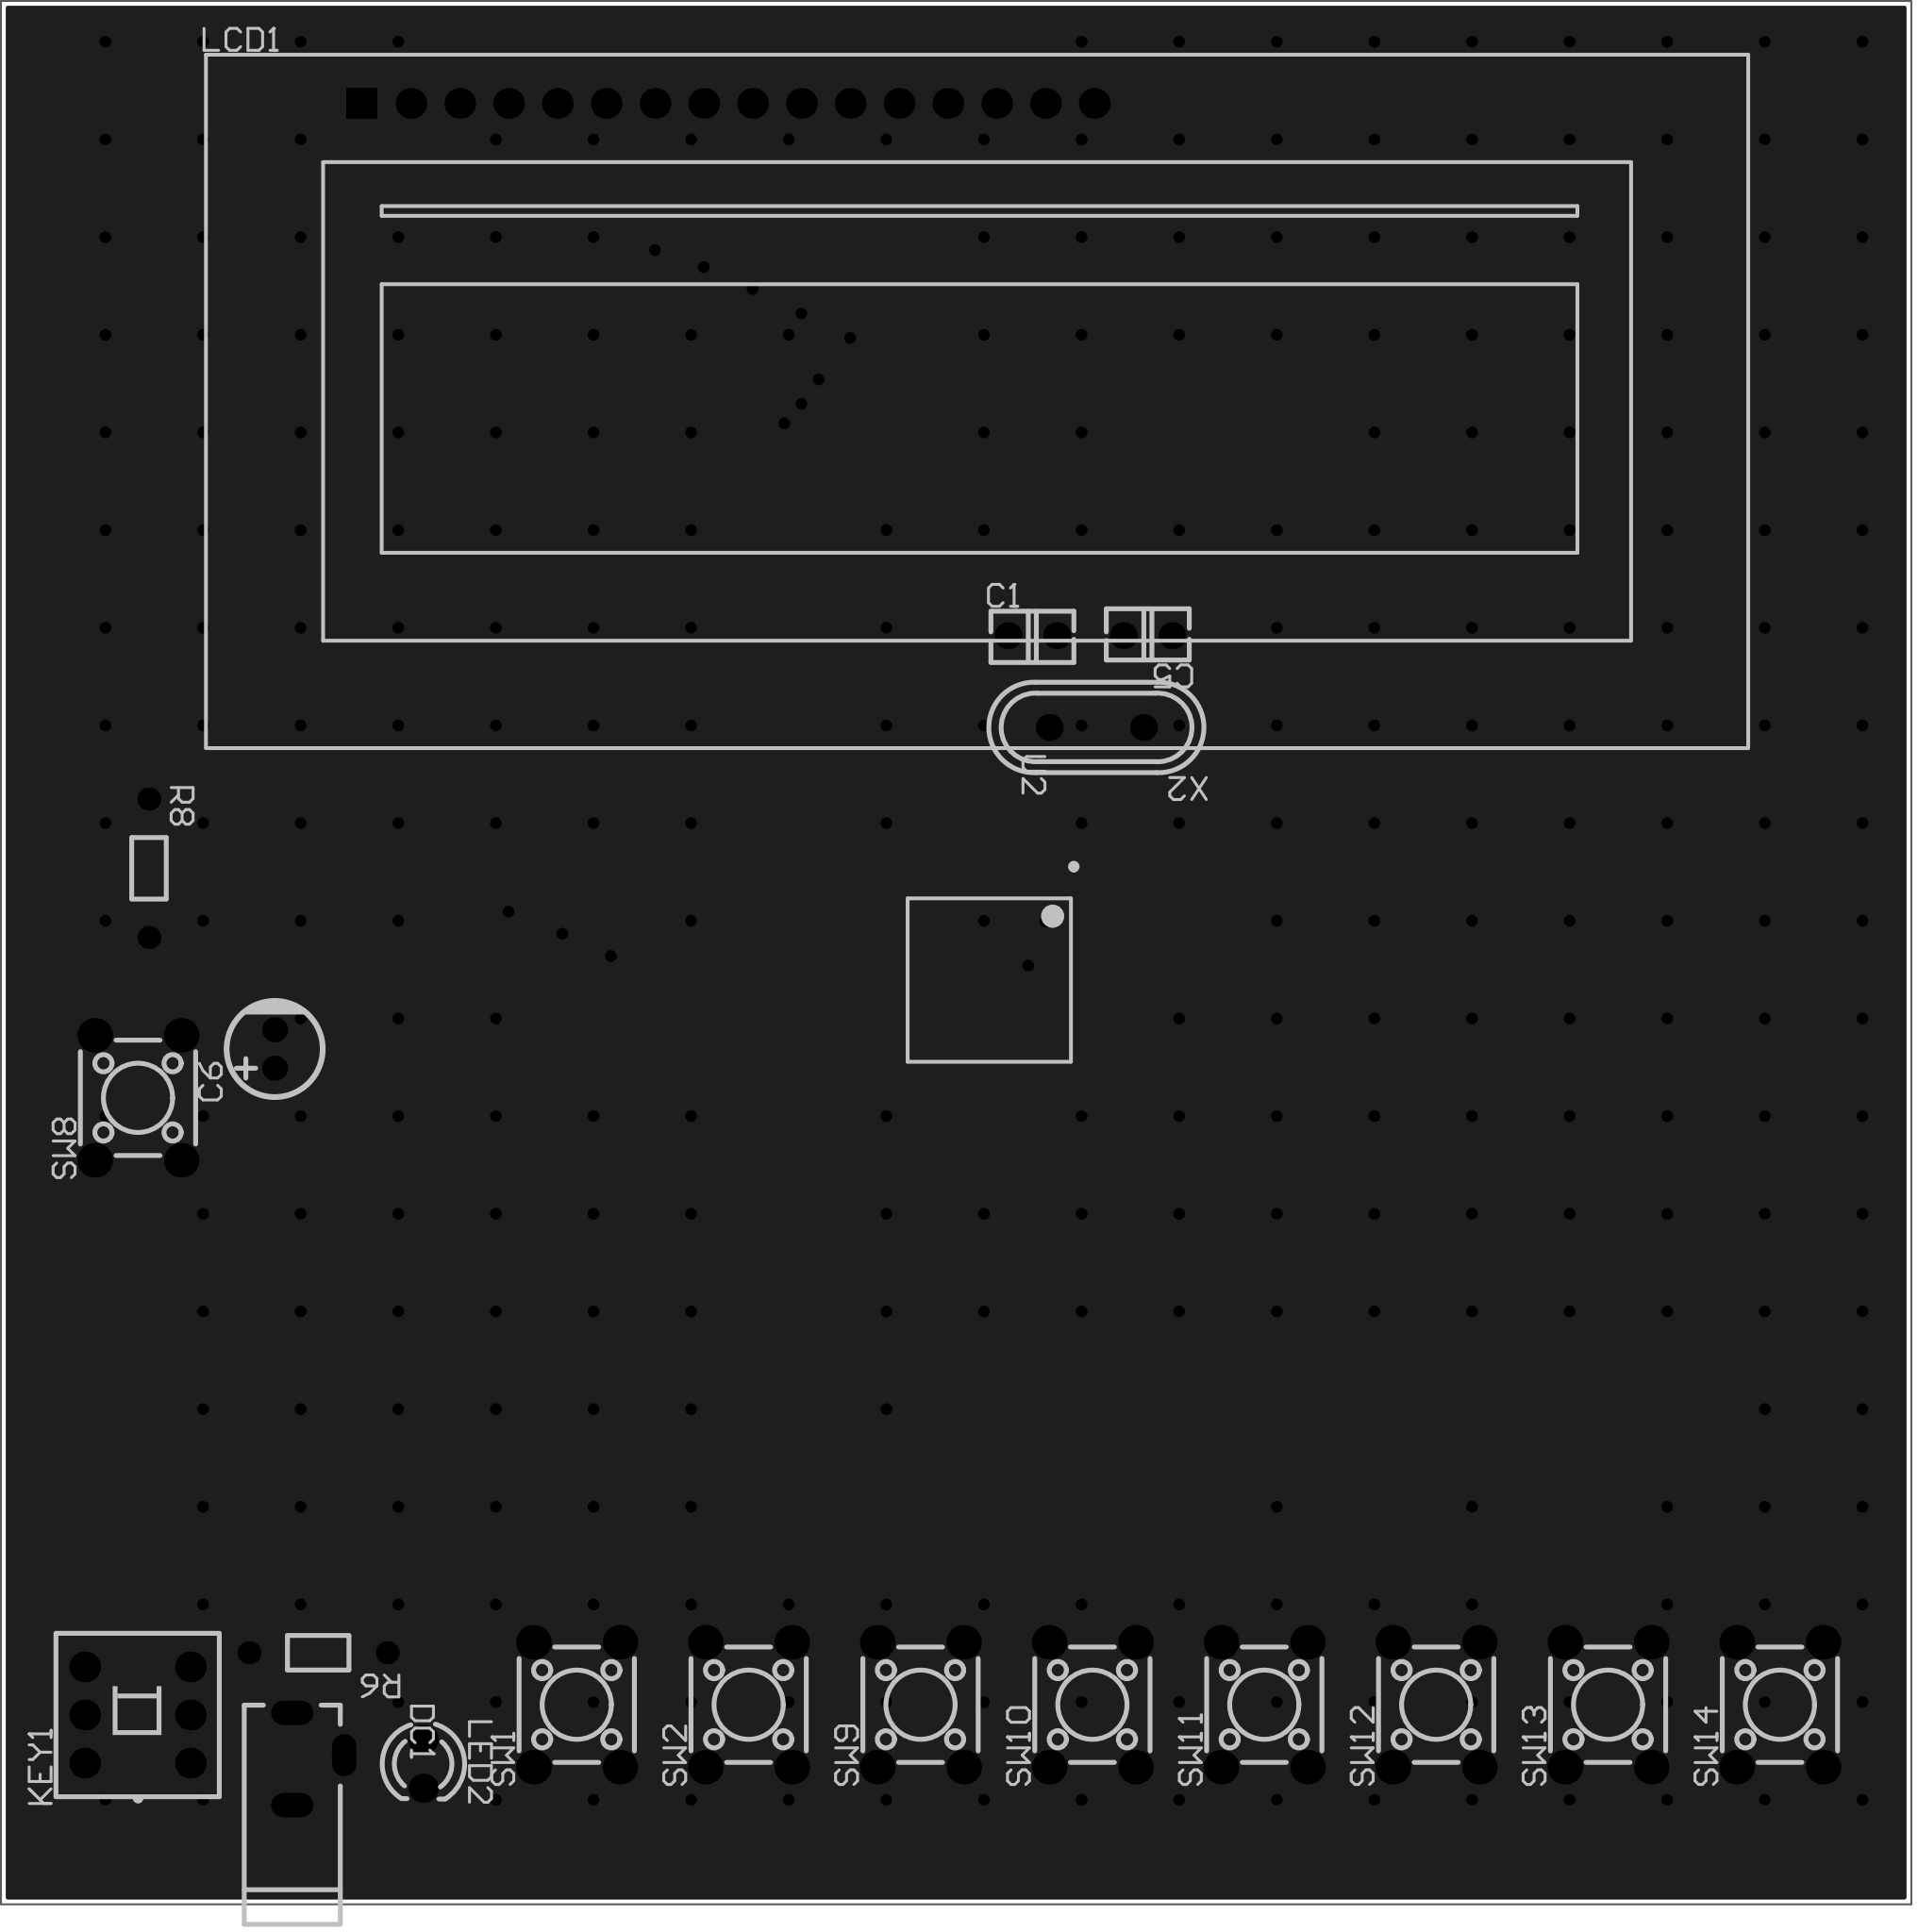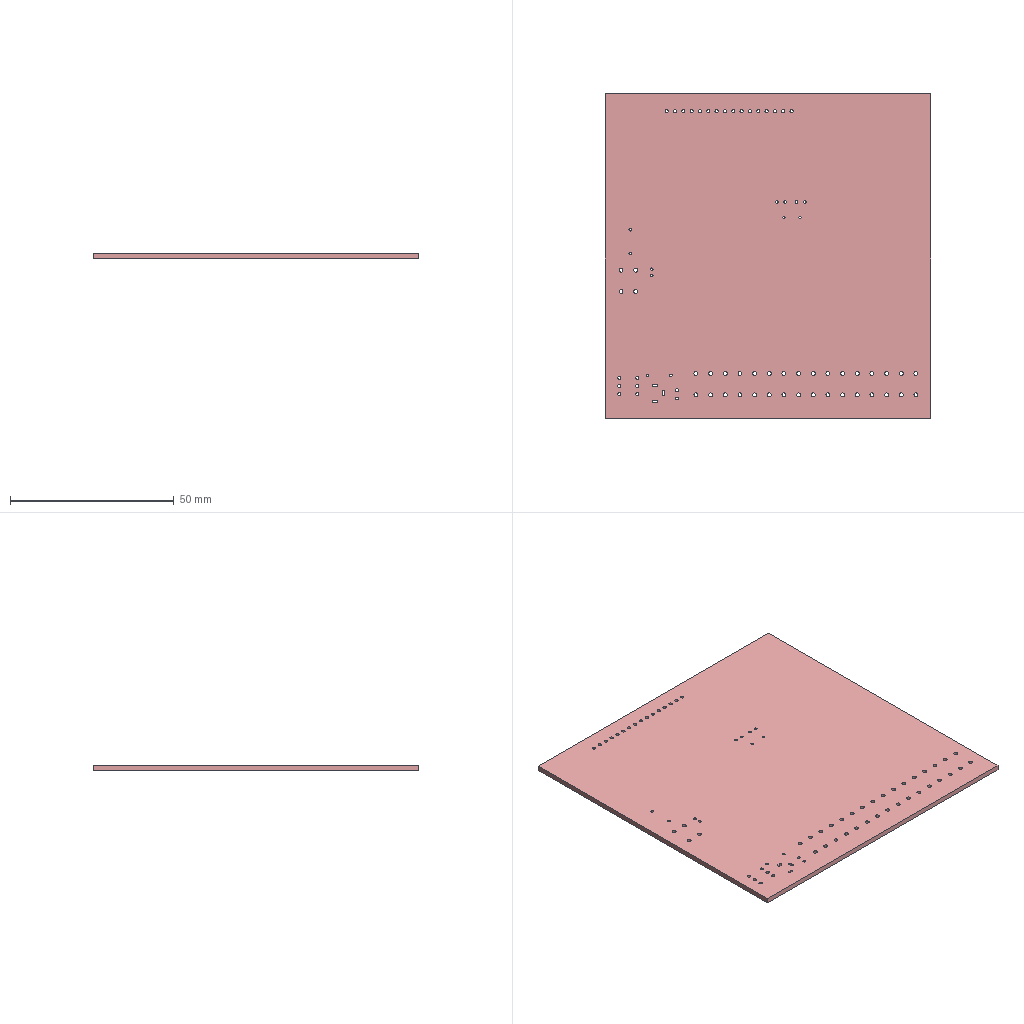Circuit board layout | Altium Designer | box 99.4 x 99 x 1.6 mm
Layer stack:
# Altium Designer layer stack of  (unit mm; dielectric type: 0 none, 1 core, 2 prepreg, 3 surface material)
index,name,kind,layer,copper_thickness_mm,dielectric_type,dielectric_thickness_mm,dielectric_material,dielectric_constant
0,Top Paste Mask Layer,other,,,,,,
1,Top Silkscreen Layer,other,,,,,,
2,Top Solder Mask Layer,dielectric,,,3,0.01,,3.3
3,Top Layer,copper,Top Layer,0.035,,,,
4,Dielectric1,dielectric,,,3,1.51,FR4,4.5
5,Bottom Layer,copper,Bottom Layer,0.035,,,,
6,Bottom Solder Mask Layer,dielectric,,,3,0.01,,3.3
7,Bottom Silkscreen Layer,other,,,,,,
8,Bottom Paste Mask Layer,other,,,,,,
# drill layer pairs: low layer,high layer
drill_pair,Top Layer,Bottom Layer
Part placement:
Designator,Comment,Layer,Footprint,Center-X(mm),Center-Y(mm),Rotation
C5,30pF,TopLayer,CAP-TH_L3.8-W2.5-P2.54-D0.50,147.187,159.776,180
C6,10uF,TopLayer,CAP-TH_BD5.0-P2.00-D0.8-FD-10UF50VC110GL,101.747,138.275,90
KEY1,Non-latching switch 8.5×8.5 silent,TopLayer,SW-TH_6P-L8.5-W8.5-P2.54,94.615,103.632,90
LCD1,LCD1602,TopLayer,LCD1602,125.353,187.458,0
LED2,,TopLayer,LED_TH-3mm,109.474,101.092,270
R8,10kΩ,TopLayer,Res_1/8W,95.206,147.673,270
R6,1kΩ,TopLayer,Res_1/8W,104.013,106.871,180
SW8,,TopLayer,SW-TH_4P-L6.0-W6.0-P4.50-LS6.5,94.635,135.735,90
SW9,,TopLayer,SW-TH_4P-L6.0-W6.0-P4.50-LS6.5,135.359,104.169,90
SW10,,TopLayer,SW-TH_4P-L6.0-W6.0-P4.50-LS6.5,144.304,104.169,90
SW11,,TopLayer,SW-TH_4P-L6.0-W6.0-P4.50-LS6.5,153.25,104.169,90
SW12,,TopLayer,SW-TH_4P-L6.0-W6.0-P4.50-LS6.5,162.195,104.169,90
SW13,,TopLayer,SW-TH_4P-L6.0-W6.0-P4.50-LS6.5,171.141,104.169,90
SW14,,TopLayer,SW-TH_4P-L6.0-W6.0-P4.50-LS6.5,180.086,104.169,90
X2,11.059MHz,TopLayer,OSC-TH_L11.1-W4.7-P4.88,144.514,155,180
DC1,DC-002,TopLayer,DC-IN-TH_DC-3510,104.013,101.346,270
SW1,,TopLayer,SW-TH_4P-L6.0-W6.0-P4.50-LS6.5,117.468,104.169,90
SW2,,TopLayer,SW-TH_4P-L6.0-W6.0-P4.50-LS6.5,126.413,104.169,90
C1,30pF,TopLayer,CAP-TH_L3.8-W2.5-P2.54-D0.50,141.182,159.776,0
U2,MSP430F2491TPM,TopLayer,LQFP-64_L10.0-W10.0-P0.50-LS12.0-TL,138.938,141.859,270
Pad and via stacks:
# Altium Designer via and pad stacks of  (unit mm). Each distinct definition once, with the count of objects using it.
# via: kind,start_layer,end_layer,hole_mm,diameter_mm,mode(0 simple;1 top-mid-bottom;2 full stack),diameter_per_layer,count,example_net
# pad: kind,layer,hole_mm,hole_type(0 round;1 square;2 slot),plating,top_size,top_shape(1 round;2 rect;3 octagon;9 rounded rect),mid_size,bottom_size,mode,footprint,size_per_layer,count,example
pad,Multi-Layer,0.8,0,plated,1.4x1.4,1,1.4x1.4,1.4x1.4,0,CAP-TH_L3.8-W2.5-P2.54-D0.50,,4,C5.1
pad,Multi-Layer,0.8,0,plated,1.3x1.3,1,1.3x1.3,1.3x1.3,0,CAP-TH_BD5.0-P2.00-D0.8-FD-10UF50VC110GL,,2,C6.2
pad,Multi-Layer,1,0,plated,1.6x1.6,1,1.6x1.6,1.6x1.6,0,SW-TH_6P-L8.5-W8.5-P2.54,,6,KEY1.4
pad,Multi-Layer,1,0,plated,1.6x1.6,1,1.6x1.6,1.6x1.6,0,LCD1602,,15,LCD1.16
pad,Multi-Layer,1,0,plated,1.6x1.6,2,1.6x1.6,1.6x1.6,0,LCD1602,,1,LCD1.1
pad,Multi-Layer,0.9144,0,plated,1.524x1.524,1,1.524x1.524,1.524x1.524,0,LED_TH-3mm,,2,LED2.1
pad,Multi-Layer,0.8001,0,plated,1.199x1.199,1,1.199x1.199,1.199x1.199,0,Res_1/8W,,4,R8.1
pad,Multi-Layer,1.2,0,plated,1.8x1.8,1,1.8x1.8,1.8x1.8,0,SW-TH_4P-L6.0-W6.0-P4.50-LS6.5,,36,SW8.1
pad,Multi-Layer,0.7,0,plated,1.4x1.4,1,1.4x1.4,1.4x1.4,0,OSC-TH_L11.1-W4.7-P4.88,,2,X2.1
pad,Multi-Layer,0.8,2,plated,2.2x1.27,1,2.2x1.27,2.2x1.27,0,DC-IN-TH_DC-3510,,3,DC1.3
pad,Top Layer,0,0,plated,0.28x1.8,1,0.28x1.8,0.28x1.8,0,LQFP-64_L10.0-W10.0-P0.50-LS12.0-TL,,32,U2.64
pad,Top Layer,0,0,plated,1.8x0.28,1,1.8x0.28,1.8x0.28,0,LQFP-64_L10.0-W10.0-P0.50-LS12.0-TL,,32,U2.48
via,Top Layer,Bottom Layer,0.3048,0.61,0,,306,P10
Copper pours:
name,layer,net,type(0 solid;1 hatched;2 none)
Top Layer-GND,Top Layer,GND,0
Bottom Layer-GND,Bottom Layer,GND,0
Design rules, without the lines most boards share:
# Altium Designer design rules of  (exported by Altium Designer, unit mm)
# columns: name | kind | enabled | priority | scope1 | scope2 | descriptor | typed fields (field=value)
creepage | 65 | enabled | 1 | All | All | Creepage Distance Constraint =(0mil) (All),(All) |